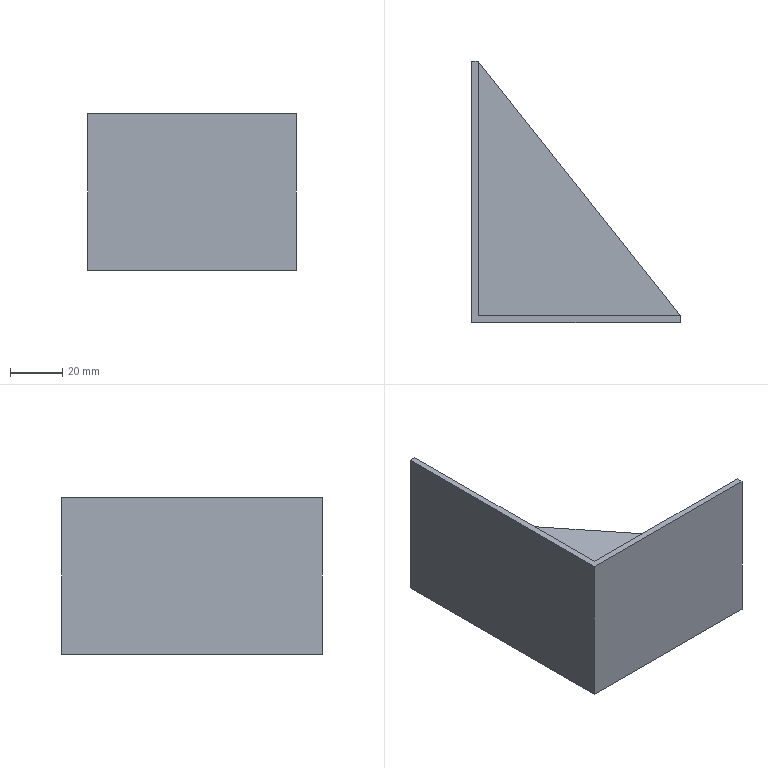Part | NX | features BREP 1 | 1 solid | 13 faces | box 80 x 100 x 60 mm | volume 36070 mm3 | plane 13
STEP:
#1=CARTESIAN_POINT('',(0.,0.,30.));
#2=VERTEX_POINT('',#1);
#3=CARTESIAN_POINT('',(0.,0.,-30.));
#4=VERTEX_POINT('',#3);
#5=CARTESIAN_POINT('',(0.,0.,30.));
#6=DIRECTION('',(0.,0.,-1.));
#7=VECTOR('',#6,1000.);
#8=LINE('',#5,#7);
#9=EDGE_CURVE('',#2,#4,#8,.T.);
#10=ORIENTED_EDGE('',*,*,#9,.F.);
#11=CARTESIAN_POINT('',(0.,100.,30.));
#12=VERTEX_POINT('',#11);
#13=CARTESIAN_POINT('',(0.,0.,30.));
#14=DIRECTION('',(0.,-1.,0.));
#15=VECTOR('',#14,1000.);
#16=LINE('',#13,#15);
#17=EDGE_CURVE('',#12,#2,#16,.T.);
#18=ORIENTED_EDGE('',*,*,#17,.F.);
#19=CARTESIAN_POINT('',(0.,100.,-30.));
#20=VERTEX_POINT('',#19);
#21=CARTESIAN_POINT('',(0.,100.,30.));
#22=DIRECTION('',(0.,0.,1.));
#23=VECTOR('',#22,1000.);
#24=LINE('',#21,#23);
#25=EDGE_CURVE('',#20,#12,#24,.T.);
#26=ORIENTED_EDGE('',*,*,#25,.F.);
#27=CARTESIAN_POINT('',(0.,0.,-30.));
#28=DIRECTION('',(0.,1.,0.));
#29=VECTOR('',#28,1000.);
#30=LINE('',#27,#29);
#31=EDGE_CURVE('',#4,#20,#30,.T.);
#32=ORIENTED_EDGE('',*,*,#31,.F.);
#33=EDGE_LOOP('',(#10,#18,#26,#32));
#34=FACE_BOUND('',#33,.T.);
#35=CARTESIAN_POINT('',(0.,0.,30.));
#36=DIRECTION('',(1.,0.,0.));
#37=DIRECTION('',(0.,1.,0.));
#38=AXIS2_PLACEMENT_3D('',#35,#36,#37);
#39=PLANE('',#38);
#40=ADVANCED_FACE('',(#34),#39,.F.);
#41=CARTESIAN_POINT('',(80.,2.5,-30.));
#42=VERTEX_POINT('',#41);
#43=CARTESIAN_POINT('',(80.,0.,-30.));
#44=VERTEX_POINT('',#43);
#45=CARTESIAN_POINT('',(80.,100.,-30.));
#46=DIRECTION('',(0.,-1.,0.));
#47=VECTOR('',#46,1000.);
#48=LINE('',#45,#47);
#49=EDGE_CURVE('',#42,#44,#48,.T.);
#50=ORIENTED_EDGE('',*,*,#49,.T.);
#51=CARTESIAN_POINT('',(0.,0.,-30.));
#52=DIRECTION('',(-1.,0.,0.));
#53=VECTOR('',#52,1000.);
#54=LINE('',#51,#53);
#55=EDGE_CURVE('',#44,#4,#54,.T.);
#56=ORIENTED_EDGE('',*,*,#55,.T.);
#57=ORIENTED_EDGE('',*,*,#31,.T.);
#58=CARTESIAN_POINT('',(2.5,100.,-30.));
#59=VERTEX_POINT('',#58);
#60=CARTESIAN_POINT('',(0.,100.,-30.));
#61=DIRECTION('',(1.,0.,0.));
#62=VECTOR('',#61,1000.);
#63=LINE('',#60,#62);
#64=EDGE_CURVE('',#20,#59,#63,.T.);
#65=ORIENTED_EDGE('',*,*,#64,.T.);
#66=CARTESIAN_POINT('',(2.5,2.5,-30.));
#67=VERTEX_POINT('',#66);
#68=CARTESIAN_POINT('',(2.5,100.,-30.));
#69=DIRECTION('',(0.,-1.,0.));
#70=VECTOR('',#69,1000.);
#71=LINE('',#68,#70);
#72=EDGE_CURVE('',#59,#67,#71,.T.);
#73=ORIENTED_EDGE('',*,*,#72,.T.);
#74=CARTESIAN_POINT('',(0.,2.5,-30.));
#75=DIRECTION('',(1.,0.,0.));
#76=VECTOR('',#75,1000.);
#77=LINE('',#74,#76);
#78=EDGE_CURVE('',#67,#42,#77,.T.);
#79=ORIENTED_EDGE('',*,*,#78,.T.);
#80=EDGE_LOOP('',(#50,#56,#57,#65,#73,#79));
#81=FACE_BOUND('',#80,.T.);
#82=CARTESIAN_POINT('',(0.,100.,-30.));
#83=DIRECTION('',(0.,0.,-1.));
#84=DIRECTION('',(0.,-1.,0.));
#85=AXIS2_PLACEMENT_3D('',#82,#83,#84);
#86=PLANE('',#85);
#87=ADVANCED_FACE('',(#81),#86,.T.);
#88=CARTESIAN_POINT('',(80.,0.,30.));
#89=VERTEX_POINT('',#88);
#90=CARTESIAN_POINT('',(80.,0.,30.));
#91=DIRECTION('',(0.,0.,-1.));
#92=VECTOR('',#91,1000.);
#93=LINE('',#90,#92);
#94=EDGE_CURVE('',#89,#44,#93,.T.);
#95=ORIENTED_EDGE('',*,*,#94,.F.);
#96=CARTESIAN_POINT('',(0.,0.,30.));
#97=DIRECTION('',(1.,0.,0.));
#98=VECTOR('',#97,1000.);
#99=LINE('',#96,#98);
#100=EDGE_CURVE('',#2,#89,#99,.T.);
#101=ORIENTED_EDGE('',*,*,#100,.F.);
#102=ORIENTED_EDGE('',*,*,#9,.T.);
#103=ORIENTED_EDGE('',*,*,#55,.F.);
#104=EDGE_LOOP('',(#95,#101,#102,#103));
#105=FACE_BOUND('',#104,.T.);
#106=CARTESIAN_POINT('',(0.,0.,30.));
#107=DIRECTION('',(0.,1.,0.));
#108=DIRECTION('',(1.,0.,0.));
#109=AXIS2_PLACEMENT_3D('',#106,#107,#108);
#110=PLANE('',#109);
#111=ADVANCED_FACE('',(#105),#110,.F.);
#112=ORIENTED_EDGE('',*,*,#100,.T.);
#113=CARTESIAN_POINT('',(80.,2.5,30.));
#114=VERTEX_POINT('',#113);
#115=CARTESIAN_POINT('',(80.,100.,30.));
#116=DIRECTION('',(0.,-1.,0.));
#117=VECTOR('',#116,1000.);
#118=LINE('',#115,#117);
#119=EDGE_CURVE('',#114,#89,#118,.T.);
#120=ORIENTED_EDGE('',*,*,#119,.F.);
#121=CARTESIAN_POINT('',(2.5,2.5,30.));
#122=VERTEX_POINT('',#121);
#123=CARTESIAN_POINT('',(0.,2.5,30.));
#124=DIRECTION('',(1.,0.,0.));
#125=VECTOR('',#124,1000.);
#126=LINE('',#123,#125);
#127=EDGE_CURVE('',#122,#114,#126,.T.);
#128=ORIENTED_EDGE('',*,*,#127,.F.);
#129=CARTESIAN_POINT('',(2.5,100.,30.));
#130=VERTEX_POINT('',#129);
#131=CARTESIAN_POINT('',(2.5,100.,30.));
#132=DIRECTION('',(0.,-1.,0.));
#133=VECTOR('',#132,1000.);
#134=LINE('',#131,#133);
#135=EDGE_CURVE('',#130,#122,#134,.T.);
#136=ORIENTED_EDGE('',*,*,#135,.F.);
#137=CARTESIAN_POINT('',(0.,100.,30.));
#138=DIRECTION('',(1.,0.,0.));
#139=VECTOR('',#138,1000.);
#140=LINE('',#137,#139);
#141=EDGE_CURVE('',#12,#130,#140,.T.);
#142=ORIENTED_EDGE('',*,*,#141,.F.);
#143=ORIENTED_EDGE('',*,*,#17,.T.);
#144=EDGE_LOOP('',(#112,#120,#128,#136,#142,#143));
#145=FACE_BOUND('',#144,.T.);
#146=CARTESIAN_POINT('',(0.,100.,30.));
#147=DIRECTION('',(0.,0.,-1.));
#148=DIRECTION('',(0.,-1.,0.));
#149=AXIS2_PLACEMENT_3D('',#146,#147,#148);
#150=PLANE('',#149);
#151=ADVANCED_FACE('',(#145),#150,.F.);
#152=ORIENTED_EDGE('',*,*,#25,.T.);
#153=ORIENTED_EDGE('',*,*,#141,.T.);
#154=CARTESIAN_POINT('',(2.5,100.,1.25));
#155=VERTEX_POINT('',#154);
#156=CARTESIAN_POINT('',(2.5,100.,30.));
#157=DIRECTION('',(0.,0.,1.));
#158=VECTOR('',#157,1000.);
#159=LINE('',#156,#158);
#160=EDGE_CURVE('',#155,#130,#159,.T.);
#161=ORIENTED_EDGE('',*,*,#160,.F.);
#162=CARTESIAN_POINT('',(2.5,100.,-1.25));
#163=VERTEX_POINT('',#162);
#164=CARTESIAN_POINT('',(2.5,100.,30.));
#165=DIRECTION('',(0.,0.,1.));
#166=VECTOR('',#165,1000.);
#167=LINE('',#164,#166);
#168=EDGE_CURVE('',#163,#155,#167,.T.);
#169=ORIENTED_EDGE('',*,*,#168,.F.);
#170=CARTESIAN_POINT('',(2.5,100.,30.));
#171=DIRECTION('',(0.,0.,1.));
#172=VECTOR('',#171,1000.);
#173=LINE('',#170,#172);
#174=EDGE_CURVE('',#59,#163,#173,.T.);
#175=ORIENTED_EDGE('',*,*,#174,.F.);
#176=ORIENTED_EDGE('',*,*,#64,.F.);
#177=EDGE_LOOP('',(#152,#153,#161,#169,#175,#176));
#178=FACE_BOUND('',#177,.T.);
#179=CARTESIAN_POINT('',(0.,100.,30.));
#180=DIRECTION('',(0.,-1.,0.));
#181=DIRECTION('',(0.,0.,-1.));
#182=AXIS2_PLACEMENT_3D('',#179,#180,#181);
#183=PLANE('',#182);
#184=ADVANCED_FACE('',(#178),#183,.F.);
#185=CARTESIAN_POINT('',(80.,2.5,-1.25));
#186=VERTEX_POINT('',#185);
#187=CARTESIAN_POINT('',(80.,2.5,30.));
#188=DIRECTION('',(0.,0.,-1.));
#189=VECTOR('',#188,1000.);
#190=LINE('',#187,#189);
#191=EDGE_CURVE('',#186,#42,#190,.T.);
#192=ORIENTED_EDGE('',*,*,#191,.F.);
#193=CARTESIAN_POINT('',(80.,2.5,1.25));
#194=VERTEX_POINT('',#193);
#195=CARTESIAN_POINT('',(80.,2.5,30.));
#196=DIRECTION('',(0.,0.,-1.));
#197=VECTOR('',#196,1000.);
#198=LINE('',#195,#197);
#199=EDGE_CURVE('',#194,#186,#198,.T.);
#200=ORIENTED_EDGE('',*,*,#199,.F.);
#201=CARTESIAN_POINT('',(80.,2.5,30.));
#202=DIRECTION('',(0.,0.,-1.));
#203=VECTOR('',#202,1000.);
#204=LINE('',#201,#203);
#205=EDGE_CURVE('',#114,#194,#204,.T.);
#206=ORIENTED_EDGE('',*,*,#205,.F.);
#207=ORIENTED_EDGE('',*,*,#119,.T.);
#208=ORIENTED_EDGE('',*,*,#94,.T.);
#209=ORIENTED_EDGE('',*,*,#49,.F.);
#210=EDGE_LOOP('',(#192,#200,#206,#207,#208,#209));
#211=FACE_BOUND('',#210,.T.);
#212=CARTESIAN_POINT('',(80.,0.,30.));
#213=DIRECTION('',(-1.,0.,0.));
#214=DIRECTION('',(0.,0.,1.));
#215=AXIS2_PLACEMENT_3D('',#212,#213,#214);
#216=PLANE('',#215);
#217=ADVANCED_FACE('',(#211),#216,.F.);
#218=CARTESIAN_POINT('',(2.5,2.5,-1.25));
#219=VERTEX_POINT('',#218);
#220=CARTESIAN_POINT('',(2.5,2.5,-1.25));
#221=DIRECTION('',(-1.,0.,0.));
#222=VECTOR('',#221,1000.);
#223=LINE('',#220,#222);
#224=EDGE_CURVE('',#186,#219,#223,.T.);
#225=ORIENTED_EDGE('',*,*,#224,.F.);
#226=ORIENTED_EDGE('',*,*,#191,.T.);
#227=ORIENTED_EDGE('',*,*,#78,.F.);
#228=CARTESIAN_POINT('',(2.5,2.5,30.));
#229=DIRECTION('',(0.,0.,-1.));
#230=VECTOR('',#229,1000.);
#231=LINE('',#228,#230);
#232=EDGE_CURVE('',#219,#67,#231,.T.);
#233=ORIENTED_EDGE('',*,*,#232,.F.);
#234=EDGE_LOOP('',(#225,#226,#227,#233));
#235=FACE_BOUND('',#234,.T.);
#236=CARTESIAN_POINT('',(2.5,2.5,30.));
#237=DIRECTION('',(0.,-1.,0.));
#238=DIRECTION('',(0.,0.,-1.));
#239=AXIS2_PLACEMENT_3D('',#236,#237,#238);
#240=PLANE('',#239);
#241=ADVANCED_FACE('',(#235),#240,.F.);
#242=CARTESIAN_POINT('',(2.5,100.,-1.25));
#243=DIRECTION('',(0.,1.,0.));
#244=VECTOR('',#243,1000.);
#245=LINE('',#242,#244);
#246=EDGE_CURVE('',#219,#163,#245,.T.);
#247=ORIENTED_EDGE('',*,*,#246,.F.);
#248=ORIENTED_EDGE('',*,*,#232,.T.);
#249=ORIENTED_EDGE('',*,*,#72,.F.);
#250=ORIENTED_EDGE('',*,*,#174,.T.);
#251=EDGE_LOOP('',(#247,#248,#249,#250));
#252=FACE_BOUND('',#251,.T.);
#253=CARTESIAN_POINT('',(2.5,100.,30.));
#254=DIRECTION('',(-1.,0.,0.));
#255=DIRECTION('',(0.,1.,0.));
#256=AXIS2_PLACEMENT_3D('',#253,#254,#255);
#257=PLANE('',#256);
#258=ADVANCED_FACE('',(#252),#257,.F.);
#259=CARTESIAN_POINT('',(2.5,2.5,1.25));
#260=VERTEX_POINT('',#259);
#261=CARTESIAN_POINT('',(2.5,2.5,30.));
#262=DIRECTION('',(0.,0.,-1.));
#263=VECTOR('',#262,1000.);
#264=LINE('',#261,#263);
#265=EDGE_CURVE('',#122,#260,#264,.T.);
#266=ORIENTED_EDGE('',*,*,#265,.F.);
#267=ORIENTED_EDGE('',*,*,#127,.T.);
#268=ORIENTED_EDGE('',*,*,#205,.T.);
#269=CARTESIAN_POINT('',(2.5,2.5,1.25));
#270=DIRECTION('',(1.,0.,0.));
#271=VECTOR('',#270,1000.);
#272=LINE('',#269,#271);
#273=EDGE_CURVE('',#260,#194,#272,.T.);
#274=ORIENTED_EDGE('',*,*,#273,.F.);
#275=EDGE_LOOP('',(#266,#267,#268,#274));
#276=FACE_BOUND('',#275,.T.);
#277=CARTESIAN_POINT('',(2.5,2.5,30.));
#278=DIRECTION('',(0.,-1.,0.));
#279=DIRECTION('',(0.,0.,-1.));
#280=AXIS2_PLACEMENT_3D('',#277,#278,#279);
#281=PLANE('',#280);
#282=ADVANCED_FACE('',(#276),#281,.F.);
#283=ORIENTED_EDGE('',*,*,#160,.T.);
#284=ORIENTED_EDGE('',*,*,#135,.T.);
#285=ORIENTED_EDGE('',*,*,#265,.T.);
#286=CARTESIAN_POINT('',(2.5,100.,1.25));
#287=DIRECTION('',(0.,-1.,0.));
#288=VECTOR('',#287,1000.);
#289=LINE('',#286,#288);
#290=EDGE_CURVE('',#155,#260,#289,.T.);
#291=ORIENTED_EDGE('',*,*,#290,.F.);
#292=EDGE_LOOP('',(#283,#284,#285,#291));
#293=FACE_BOUND('',#292,.T.);
#294=CARTESIAN_POINT('',(2.5,100.,30.));
#295=DIRECTION('',(-1.,0.,0.));
#296=DIRECTION('',(0.,1.,0.));
#297=AXIS2_PLACEMENT_3D('',#294,#295,#296);
#298=PLANE('',#297);
#299=ADVANCED_FACE('',(#293),#298,.F.);
#300=ORIENTED_EDGE('',*,*,#168,.T.);
#301=CARTESIAN_POINT('',(80.,2.5,1.25));
#302=DIRECTION('',(-0.6222,0.7828,0.));
#303=VECTOR('',#302,1000.);
#304=LINE('',#301,#303);
#305=EDGE_CURVE('',#194,#155,#304,.T.);
#306=ORIENTED_EDGE('',*,*,#305,.F.);
#307=ORIENTED_EDGE('',*,*,#199,.T.);
#308=CARTESIAN_POINT('',(80.,2.5,-1.25));
#309=DIRECTION('',(0.6222,-0.7828,0.));
#310=VECTOR('',#309,1000.);
#311=LINE('',#308,#310);
#312=EDGE_CURVE('',#163,#186,#311,.T.);
#313=ORIENTED_EDGE('',*,*,#312,.F.);
#314=EDGE_LOOP('',(#300,#306,#307,#313));
#315=FACE_BOUND('',#314,.T.);
#316=CARTESIAN_POINT('',(80.,2.5,1.25));
#317=DIRECTION('',(-0.7828,-0.6222,0.));
#318=DIRECTION('',(-0.6222,0.7828,0.));
#319=AXIS2_PLACEMENT_3D('',#316,#317,#318);
#320=PLANE('',#319);
#321=ADVANCED_FACE('',(#315),#320,.F.);
#322=ORIENTED_EDGE('',*,*,#224,.T.);
#323=ORIENTED_EDGE('',*,*,#246,.T.);
#324=ORIENTED_EDGE('',*,*,#312,.T.);
#325=EDGE_LOOP('',(#322,#323,#324));
#326=FACE_BOUND('',#325,.T.);
#327=CARTESIAN_POINT('',(80.,2.5,-1.25));
#328=DIRECTION('',(0.,0.,-1.));
#329=DIRECTION('',(0.,-1.,0.));
#330=AXIS2_PLACEMENT_3D('',#327,#328,#329);
#331=PLANE('',#330);
#332=ADVANCED_FACE('',(#326),#331,.T.);
#333=ORIENTED_EDGE('',*,*,#290,.T.);
#334=ORIENTED_EDGE('',*,*,#273,.T.);
#335=ORIENTED_EDGE('',*,*,#305,.T.);
#336=EDGE_LOOP('',(#333,#334,#335));
#337=FACE_BOUND('',#336,.T.);
#338=CARTESIAN_POINT('',(80.,2.5,1.25));
#339=DIRECTION('',(0.,0.,-1.));
#340=DIRECTION('',(0.,-1.,0.));
#341=AXIS2_PLACEMENT_3D('',#338,#339,#340);
#342=PLANE('',#341);
#343=ADVANCED_FACE('',(#337),#342,.F.);
#344=CLOSED_SHELL('',(#40,#87,#111,#151,#184,#217,#241,#258,#282,#299,#321,#332,#343));
#345=MANIFOLD_SOLID_BREP('',#344);
#346=(LENGTH_UNIT()NAMED_UNIT(*)SI_UNIT(.MILLI.,.METRE.));
#347=UNCERTAINTY_MEASURE_WITH_UNIT(LENGTH_MEASURE(0.00001),#346,'','');
#348=(NAMED_UNIT(*)PLANE_ANGLE_UNIT()SI_UNIT($,.RADIAN.));
#349=(NAMED_UNIT(*)SI_UNIT($,.STERADIAN.)SOLID_ANGLE_UNIT());
#350=(GEOMETRIC_REPRESENTATION_CONTEXT(3)GLOBAL_UNCERTAINTY_ASSIGNED_CONTEXT((#347))GLOBAL_UNIT_ASSIGNED_CONTEXT((#346,#348,#349))REPRESENTATION_CONTEXT('',''));
#351=ADVANCED_BREP_SHAPE_REPRESENTATION('',(#345),#350);